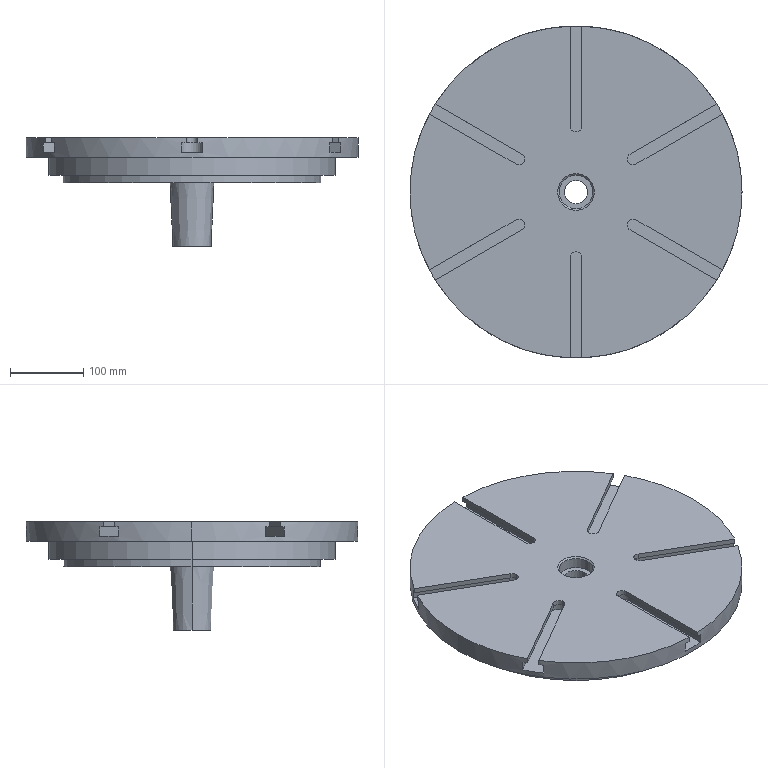Part | SolidWorks | features Cut 2, ICE 2, Chamfer 1, CirPattern 1, Revolution 1 | 1 solid | 81 faces | box 454 x 454 x 148.4 mm | volume 7848995 mm3 | plane 45 | cylinder 32 | cone 4 | commonest cylinder face diameters 16 x8 30 x8 32 x2 46 x2 352 x2 392 x2